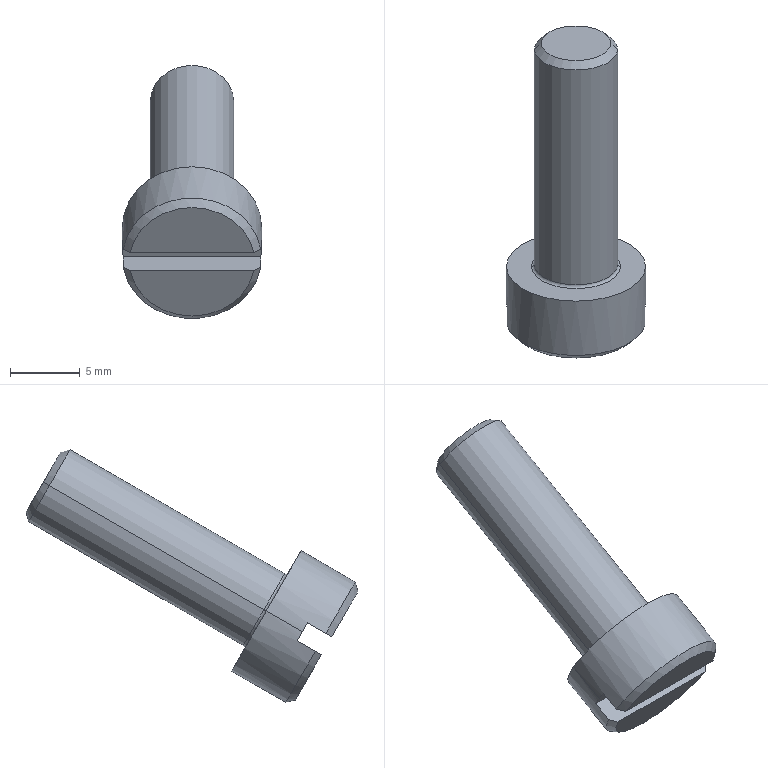Part | SolidWorks | features BaseBody 1 | 1 solid | 17 faces | box 10 x 23.852 x 18.178 mm | volume 880.406 mm3 | plane 7 | cone 4 | cylinder 4 | torus 2 | commonest cylinder face diameters 6 x2 10 x2
STEP:
#1=CARTESIAN_POINT('',(130.5,-22.084,-12.75));
#2=VERTEX_POINT('',#1);
#3=CARTESIAN_POINT('',(135.5,-22.084,-12.75));
#4=VERTEX_POINT('',#3);
#5=CARTESIAN_POINT('',(133.,-22.084,-12.75));
#6=DIRECTION('',(0.,0.866,0.5));
#7=DIRECTION('',(-1.,0.,0.));
#8=AXIS2_PLACEMENT_3D('',#5,#6,#7);
#9=CIRCLE('',#8,2.5);
#10=EDGE_CURVE('',#2,#4,#9,.T.);
#11=ORIENTED_EDGE('',*,*,#10,.F.);
#12=CARTESIAN_POINT('',(130.,-22.517,-13.));
#13=VERTEX_POINT('',#12);
#14=CARTESIAN_POINT('',(130.5,-22.084,-12.75));
#15=DIRECTION('',(-0.7071,-0.6124,-0.3536));
#16=VECTOR('',#15,1000.);
#17=LINE('',#14,#16);
#18=EDGE_CURVE('',#2,#13,#17,.T.);
#19=ORIENTED_EDGE('',*,*,#18,.T.);
#20=CARTESIAN_POINT('',(136.,-22.517,-13.));
#21=VERTEX_POINT('',#20);
#22=CARTESIAN_POINT('',(133.,-22.517,-13.));
#23=DIRECTION('',(0.,-0.866,-0.5));
#24=DIRECTION('',(-1.,0.,0.));
#25=AXIS2_PLACEMENT_3D('',#22,#23,#24);
#26=CIRCLE('',#25,3.);
#27=EDGE_CURVE('',#21,#13,#26,.T.);
#28=ORIENTED_EDGE('',*,*,#27,.F.);
#29=CARTESIAN_POINT('',(135.5,-22.084,-12.75));
#30=DIRECTION('',(0.7071,-0.6124,-0.3536));
#31=VECTOR('',#30,1000.);
#32=LINE('',#29,#31);
#33=EDGE_CURVE('',#4,#21,#32,.T.);
#34=ORIENTED_EDGE('',*,*,#33,.F.);
#35=EDGE_LOOP('',(#11,#19,#28,#34));
#36=FACE_OUTER_BOUND('',#35,.T.);
#37=CARTESIAN_POINT('',(133.,-22.084,-12.75));
#38=DIRECTION('',(0.,-0.866,-0.5));
#39=DIRECTION('',(1.,0.,0.));
#40=AXIS2_PLACEMENT_3D('',#37,#38,#39);
#41=CONICAL_SURFACE('',#40,2.5,0.7854);
#42=ADVANCED_FACE('',(#36),#41,.T.);
#43=CARTESIAN_POINT('',(136.,-37.932,-21.9));
#44=VERTEX_POINT('',#43);
#45=CARTESIAN_POINT('',(130.,-37.932,-21.9));
#46=VERTEX_POINT('',#45);
#47=CARTESIAN_POINT('',(133.,-37.932,-21.9));
#48=DIRECTION('',(0.,0.866,0.5));
#49=DIRECTION('',(-1.,0.,0.));
#50=AXIS2_PLACEMENT_3D('',#47,#48,#49);
#51=CIRCLE('',#50,3.);
#52=EDGE_CURVE('',#44,#46,#51,.T.);
#53=ORIENTED_EDGE('',*,*,#52,.F.);
#54=CARTESIAN_POINT('',(136.2,-38.105,-22.));
#55=VERTEX_POINT('',#54);
#56=CARTESIAN_POINT('',(136.2,-37.932,-21.9));
#57=DIRECTION('',(0.,-0.5,0.866));
#58=DIRECTION('',(0.,-0.866,-0.5));
#59=AXIS2_PLACEMENT_3D('',#56,#57,#58);
#60=CIRCLE('',#59,0.2);
#61=EDGE_CURVE('',#44,#55,#60,.T.);
#62=ORIENTED_EDGE('',*,*,#61,.T.);
#63=CARTESIAN_POINT('',(129.8,-38.105,-22.));
#64=VERTEX_POINT('',#63);
#65=CARTESIAN_POINT('',(133.,-38.105,-22.));
#66=DIRECTION('',(0.,-0.866,-0.5));
#67=DIRECTION('',(-1.,0.,0.));
#68=AXIS2_PLACEMENT_3D('',#65,#66,#67);
#69=CIRCLE('',#68,3.2);
#70=EDGE_CURVE('',#64,#55,#69,.T.);
#71=ORIENTED_EDGE('',*,*,#70,.F.);
#72=CARTESIAN_POINT('',(129.8,-37.932,-21.9));
#73=DIRECTION('',(0.,0.5,-0.866));
#74=DIRECTION('',(0.,0.866,0.5));
#75=AXIS2_PLACEMENT_3D('',#72,#73,#74);
#76=CIRCLE('',#75,0.2);
#77=EDGE_CURVE('',#46,#64,#76,.T.);
#78=ORIENTED_EDGE('',*,*,#77,.F.);
#79=EDGE_LOOP('',(#53,#62,#71,#78));
#80=FACE_OUTER_BOUND('',#79,.T.);
#81=CARTESIAN_POINT('',(133.,-37.932,-21.9));
#82=DIRECTION('',(0.,0.866,0.5));
#83=DIRECTION('',(-1.,0.,0.));
#84=AXIS2_PLACEMENT_3D('',#81,#82,#83);
#85=TOROIDAL_SURFACE('',#84,3.2,0.2);
#86=ADVANCED_FACE('',(#80),#85,.F.);
#87=ORIENTED_EDGE('',*,*,#27,.T.);
#88=CARTESIAN_POINT('',(130.,-22.084,-12.75));
#89=DIRECTION('',(0.,-0.866,-0.5));
#90=VECTOR('',#89,1000.);
#91=LINE('',#88,#90);
#92=EDGE_CURVE('',#13,#46,#91,.T.);
#93=ORIENTED_EDGE('',*,*,#92,.T.);
#94=CARTESIAN_POINT('',(133.,-37.932,-21.9));
#95=DIRECTION('',(0.,0.866,0.5));
#96=DIRECTION('',(-1.,0.,0.));
#97=AXIS2_PLACEMENT_3D('',#94,#95,#96);
#98=CIRCLE('',#97,3.);
#99=EDGE_CURVE('',#46,#44,#98,.T.);
#100=ORIENTED_EDGE('',*,*,#99,.T.);
#101=CARTESIAN_POINT('',(136.,-22.084,-12.75));
#102=DIRECTION('',(0.,-0.866,-0.5));
#103=VECTOR('',#102,1000.);
#104=LINE('',#101,#103);
#105=EDGE_CURVE('',#21,#44,#104,.T.);
#106=ORIENTED_EDGE('',*,*,#105,.F.);
#107=EDGE_LOOP('',(#87,#93,#100,#106));
#108=FACE_OUTER_BOUND('',#107,.T.);
#109=CARTESIAN_POINT('',(133.,-22.084,-12.75));
#110=DIRECTION('',(0.,-0.866,-0.5));
#111=DIRECTION('',(1.,0.,0.));
#112=AXIS2_PLACEMENT_3D('',#109,#110,#111);
#113=CYLINDRICAL_SURFACE('',#112,3.);
#114=ADVANCED_FACE('',(#108),#113,.T.);
#115=CARTESIAN_POINT('',(128.,-38.105,-22.));
#116=VERTEX_POINT('',#115);
#117=CARTESIAN_POINT('',(138.,-38.105,-22.));
#118=VERTEX_POINT('',#117);
#119=CARTESIAN_POINT('',(133.,-38.105,-22.));
#120=DIRECTION('',(0.,0.866,0.5));
#121=DIRECTION('',(-1.,0.,0.));
#122=AXIS2_PLACEMENT_3D('',#119,#120,#121);
#123=CIRCLE('',#122,5.);
#124=EDGE_CURVE('',#116,#118,#123,.T.);
#125=ORIENTED_EDGE('',*,*,#124,.F.);
#126=CARTESIAN_POINT('',(128.,-40.703,-23.5));
#127=VERTEX_POINT('',#126);
#128=CARTESIAN_POINT('',(128.,-38.105,-22.));
#129=DIRECTION('',(0.,-0.866,-0.5));
#130=VECTOR('',#129,1000.);
#131=LINE('',#128,#130);
#132=EDGE_CURVE('',#116,#127,#131,.T.);
#133=ORIENTED_EDGE('',*,*,#132,.T.);
#134=CARTESIAN_POINT('',(128.057,-41.078,-22.85));
#135=VERTEX_POINT('',#134);
#136=CARTESIAN_POINT('',(133.,-40.703,-23.5));
#137=DIRECTION('',(0.,-0.866,-0.5));
#138=DIRECTION('',(1.,0.,0.));
#139=AXIS2_PLACEMENT_3D('',#136,#137,#138);
#140=CIRCLE('',#139,5.);
#141=EDGE_CURVE('',#135,#127,#140,.T.);
#142=ORIENTED_EDGE('',*,*,#141,.F.);
#143=CARTESIAN_POINT('',(128.057,-42.377,-23.6));
#144=VERTEX_POINT('',#143);
#145=CARTESIAN_POINT('',(128.057,-41.078,-22.85));
#146=DIRECTION('',(0.,-0.866,-0.5));
#147=VECTOR('',#146,1000.);
#148=LINE('',#145,#147);
#149=EDGE_CURVE('',#135,#144,#148,.T.);
#150=ORIENTED_EDGE('',*,*,#149,.T.);
#151=CARTESIAN_POINT('',(137.943,-42.377,-23.6));
#152=VERTEX_POINT('',#151);
#153=CARTESIAN_POINT('',(133.,-42.002,-24.25));
#154=DIRECTION('',(0.,0.866,0.5));
#155=DIRECTION('',(-1.,0.,0.));
#156=AXIS2_PLACEMENT_3D('',#153,#154,#155);
#157=CIRCLE('',#156,5.);
#158=EDGE_CURVE('',#144,#152,#157,.T.);
#159=ORIENTED_EDGE('',*,*,#158,.T.);
#160=CARTESIAN_POINT('',(137.943,-41.078,-22.85));
#161=VERTEX_POINT('',#160);
#162=CARTESIAN_POINT('',(137.943,-41.078,-22.85));
#163=DIRECTION('',(0.,-0.866,-0.5));
#164=VECTOR('',#163,1000.);
#165=LINE('',#162,#164);
#166=EDGE_CURVE('',#161,#152,#165,.T.);
#167=ORIENTED_EDGE('',*,*,#166,.F.);
#168=CARTESIAN_POINT('',(138.,-40.703,-23.5));
#169=VERTEX_POINT('',#168);
#170=CARTESIAN_POINT('',(133.,-40.703,-23.5));
#171=DIRECTION('',(0.,-0.866,-0.5));
#172=DIRECTION('',(1.,0.,0.));
#173=AXIS2_PLACEMENT_3D('',#170,#171,#172);
#174=CIRCLE('',#173,5.);
#175=EDGE_CURVE('',#169,#161,#174,.T.);
#176=ORIENTED_EDGE('',*,*,#175,.F.);
#177=CARTESIAN_POINT('',(138.,-38.105,-22.));
#178=DIRECTION('',(0.,-0.866,-0.5));
#179=VECTOR('',#178,1000.);
#180=LINE('',#177,#179);
#181=EDGE_CURVE('',#118,#169,#180,.T.);
#182=ORIENTED_EDGE('',*,*,#181,.F.);
#183=EDGE_LOOP('',(#125,#133,#142,#150,#159,#167,#176,#182));
#184=FACE_OUTER_BOUND('',#183,.T.);
#185=CARTESIAN_POINT('',(133.,-38.105,-22.));
#186=DIRECTION('',(0.,-0.866,-0.5));
#187=DIRECTION('',(1.,0.,0.));
#188=AXIS2_PLACEMENT_3D('',#185,#186,#187);
#189=CYLINDRICAL_SURFACE('',#188,5.);
#190=ADVANCED_FACE('',(#184),#189,.T.);
#191=ORIENTED_EDGE('',*,*,#70,.T.);
#192=CARTESIAN_POINT('',(133.,-38.105,-22.));
#193=DIRECTION('',(0.,-0.866,-0.5));
#194=DIRECTION('',(-1.,0.,0.));
#195=AXIS2_PLACEMENT_3D('',#192,#193,#194);
#196=CIRCLE('',#195,3.2);
#197=EDGE_CURVE('',#55,#64,#196,.T.);
#198=ORIENTED_EDGE('',*,*,#197,.T.);
#199=EDGE_LOOP('',(#191,#198));
#200=FACE_BOUND('',#199,.T.);
#201=CARTESIAN_POINT('',(133.,-38.105,-22.));
#202=DIRECTION('',(0.,0.866,0.5));
#203=DIRECTION('',(-1.,0.,0.));
#204=AXIS2_PLACEMENT_3D('',#201,#202,#203);
#205=CIRCLE('',#204,5.);
#206=EDGE_CURVE('',#118,#116,#205,.T.);
#207=ORIENTED_EDGE('',*,*,#206,.T.);
#208=ORIENTED_EDGE('',*,*,#124,.T.);
#209=EDGE_LOOP('',(#207,#208));
#210=FACE_OUTER_BOUND('',#209,.T.);
#211=CARTESIAN_POINT('',(133.,-38.105,-22.));
#212=DIRECTION('',(0.,0.866,0.5));
#213=DIRECTION('',(-1.,0.,0.));
#214=AXIS2_PLACEMENT_3D('',#211,#212,#213);
#215=PLANE('',#214);
#216=ADVANCED_FACE('',(#200,#210),#215,.T.);
#217=CARTESIAN_POINT('',(137.437,-42.81,-23.85));
#218=VERTEX_POINT('',#217);
#219=CARTESIAN_POINT('',(128.563,-42.81,-23.85));
#220=VERTEX_POINT('',#219);
#221=CARTESIAN_POINT('',(128.057,-42.81,-23.85));
#222=DIRECTION('',(-1.,0.,0.));
#223=VECTOR('',#222,1000.);
#224=LINE('',#221,#223);
#225=EDGE_CURVE('',#218,#220,#224,.T.);
#226=ORIENTED_EDGE('',*,*,#225,.F.);
#227=CARTESIAN_POINT('',(133.,-42.435,-24.5));
#228=DIRECTION('',(0.,-0.866,-0.5));
#229=DIRECTION('',(-1.,0.,0.));
#230=AXIS2_PLACEMENT_3D('',#227,#228,#229);
#231=CIRCLE('',#230,4.5);
#232=EDGE_CURVE('',#218,#220,#231,.T.);
#233=ORIENTED_EDGE('',*,*,#232,.T.);
#234=EDGE_LOOP('',(#226,#233));
#235=FACE_OUTER_BOUND('',#234,.T.);
#236=CARTESIAN_POINT('',(133.,-42.435,-24.5));
#237=DIRECTION('',(0.,0.866,0.5));
#238=DIRECTION('',(-1.,0.,0.));
#239=AXIS2_PLACEMENT_3D('',#236,#237,#238);
#240=PLANE('',#239);
#241=ADVANCED_FACE('',(#235),#240,.F.);
#242=ORIENTED_EDGE('',*,*,#132,.F.);
#243=ORIENTED_EDGE('',*,*,#206,.F.);
#244=ORIENTED_EDGE('',*,*,#181,.T.);
#245=CARTESIAN_POINT('',(137.943,-40.328,-24.15));
#246=VERTEX_POINT('',#245);
#247=CARTESIAN_POINT('',(133.,-40.703,-23.5));
#248=DIRECTION('',(0.,-0.866,-0.5));
#249=DIRECTION('',(1.,0.,0.));
#250=AXIS2_PLACEMENT_3D('',#247,#248,#249);
#251=CIRCLE('',#250,5.);
#252=EDGE_CURVE('',#246,#169,#251,.T.);
#253=ORIENTED_EDGE('',*,*,#252,.F.);
#254=CARTESIAN_POINT('',(137.943,-41.627,-24.9));
#255=VERTEX_POINT('',#254);
#256=CARTESIAN_POINT('',(137.943,-40.328,-24.15));
#257=DIRECTION('',(0.,-0.866,-0.5));
#258=VECTOR('',#257,1000.);
#259=LINE('',#256,#258);
#260=EDGE_CURVE('',#246,#255,#259,.T.);
#261=ORIENTED_EDGE('',*,*,#260,.T.);
#262=CARTESIAN_POINT('',(128.057,-41.627,-24.9));
#263=VERTEX_POINT('',#262);
#264=CARTESIAN_POINT('',(133.,-42.002,-24.25));
#265=DIRECTION('',(0.,0.866,0.5));
#266=DIRECTION('',(-1.,0.,0.));
#267=AXIS2_PLACEMENT_3D('',#264,#265,#266);
#268=CIRCLE('',#267,5.);
#269=EDGE_CURVE('',#255,#263,#268,.T.);
#270=ORIENTED_EDGE('',*,*,#269,.T.);
#271=CARTESIAN_POINT('',(128.057,-40.328,-24.15));
#272=VERTEX_POINT('',#271);
#273=CARTESIAN_POINT('',(128.057,-40.328,-24.15));
#274=DIRECTION('',(0.,-0.866,-0.5));
#275=VECTOR('',#274,1000.);
#276=LINE('',#273,#275);
#277=EDGE_CURVE('',#272,#263,#276,.T.);
#278=ORIENTED_EDGE('',*,*,#277,.F.);
#279=CARTESIAN_POINT('',(133.,-40.703,-23.5));
#280=DIRECTION('',(0.,-0.866,-0.5));
#281=DIRECTION('',(1.,0.,0.));
#282=AXIS2_PLACEMENT_3D('',#279,#280,#281);
#283=CIRCLE('',#282,5.);
#284=EDGE_CURVE('',#127,#272,#283,.T.);
#285=ORIENTED_EDGE('',*,*,#284,.F.);
#286=EDGE_LOOP('',(#242,#243,#244,#253,#261,#270,#278,#285));
#287=FACE_OUTER_BOUND('',#286,.T.);
#288=CARTESIAN_POINT('',(133.,-38.105,-22.));
#289=DIRECTION('',(0.,-0.866,-0.5));
#290=DIRECTION('',(1.,0.,0.));
#291=AXIS2_PLACEMENT_3D('',#288,#289,#290);
#292=CYLINDRICAL_SURFACE('',#291,5.);
#293=ADVANCED_FACE('',(#287),#292,.T.);
#294=CARTESIAN_POINT('',(128.563,-42.06,-25.15));
#295=VERTEX_POINT('',#294);
#296=CARTESIAN_POINT('',(137.437,-42.06,-25.15));
#297=VERTEX_POINT('',#296);
#298=CARTESIAN_POINT('',(128.057,-42.06,-25.15));
#299=DIRECTION('',(1.,0.,0.));
#300=VECTOR('',#299,1000.);
#301=LINE('',#298,#300);
#302=EDGE_CURVE('',#295,#297,#301,.T.);
#303=ORIENTED_EDGE('',*,*,#302,.F.);
#304=CARTESIAN_POINT('',(133.,-42.435,-24.5));
#305=DIRECTION('',(0.,-0.866,-0.5));
#306=DIRECTION('',(-1.,0.,0.));
#307=AXIS2_PLACEMENT_3D('',#304,#305,#306);
#308=CIRCLE('',#307,4.5);
#309=EDGE_CURVE('',#295,#297,#308,.T.);
#310=ORIENTED_EDGE('',*,*,#309,.T.);
#311=EDGE_LOOP('',(#303,#310));
#312=FACE_OUTER_BOUND('',#311,.T.);
#313=CARTESIAN_POINT('',(133.,-42.435,-24.5));
#314=DIRECTION('',(0.,0.866,0.5));
#315=DIRECTION('',(-1.,0.,0.));
#316=AXIS2_PLACEMENT_3D('',#313,#314,#315);
#317=PLANE('',#316);
#318=ADVANCED_FACE('',(#312),#317,.F.);
#319=ORIENTED_EDGE('',*,*,#166,.T.);
#320=CARTESIAN_POINT('',(137.943,-42.377,-23.6));
#321=CARTESIAN_POINT('',(137.775,-42.522,-23.684));
#322=CARTESIAN_POINT('',(137.606,-42.666,-23.767));
#323=CARTESIAN_POINT('',(137.437,-42.81,-23.85));
#324=B_SPLINE_CURVE_WITH_KNOTS('',3,(#320,#321,#322,#323),.UNSPECIFIED.,.F.,.F.,(4,4),(0.,0.0007116),.UNSPECIFIED.);
#325=EDGE_CURVE('',#152,#218,#324,.T.);
#326=ORIENTED_EDGE('',*,*,#325,.T.);
#327=ORIENTED_EDGE('',*,*,#225,.T.);
#328=CARTESIAN_POINT('',(128.563,-42.81,-23.85));
#329=CARTESIAN_POINT('',(128.394,-42.666,-23.767));
#330=CARTESIAN_POINT('',(128.225,-42.522,-23.684));
#331=CARTESIAN_POINT('',(128.057,-42.377,-23.6));
#332=B_SPLINE_CURVE_WITH_KNOTS('',3,(#328,#329,#330,#331),.UNSPECIFIED.,.F.,.F.,(4,4),(0.,0.0007116),.UNSPECIFIED.);
#333=EDGE_CURVE('',#220,#144,#332,.T.);
#334=ORIENTED_EDGE('',*,*,#333,.T.);
#335=ORIENTED_EDGE('',*,*,#149,.F.);
#336=CARTESIAN_POINT('',(128.057,-41.078,-22.85));
#337=DIRECTION('',(-1.,0.,0.));
#338=VECTOR('',#337,1000.);
#339=LINE('',#336,#338);
#340=EDGE_CURVE('',#161,#135,#339,.T.);
#341=ORIENTED_EDGE('',*,*,#340,.F.);
#342=EDGE_LOOP('',(#319,#326,#327,#334,#335,#341));
#343=FACE_OUTER_BOUND('',#342,.T.);
#344=CARTESIAN_POINT('',(128.057,-41.078,-22.85));
#345=DIRECTION('',(0.,-0.5,0.866));
#346=DIRECTION('',(0.,0.866,0.5));
#347=AXIS2_PLACEMENT_3D('',#344,#345,#346);
#348=PLANE('',#347);
#349=ADVANCED_FACE('',(#343),#348,.F.);
#350=ORIENTED_EDGE('',*,*,#277,.T.);
#351=CARTESIAN_POINT('',(128.057,-41.627,-24.9));
#352=CARTESIAN_POINT('',(128.225,-41.772,-24.983));
#353=CARTESIAN_POINT('',(128.394,-41.916,-25.066));
#354=CARTESIAN_POINT('',(128.563,-42.06,-25.15));
#355=B_SPLINE_CURVE_WITH_KNOTS('',3,(#351,#352,#353,#354),.UNSPECIFIED.,.F.,.F.,(4,4),(0.,0.0007116),.UNSPECIFIED.);
#356=EDGE_CURVE('',#263,#295,#355,.T.);
#357=ORIENTED_EDGE('',*,*,#356,.T.);
#358=ORIENTED_EDGE('',*,*,#302,.T.);
#359=CARTESIAN_POINT('',(137.437,-42.06,-25.15));
#360=CARTESIAN_POINT('',(137.606,-41.916,-25.066));
#361=CARTESIAN_POINT('',(137.775,-41.772,-24.983));
#362=CARTESIAN_POINT('',(137.943,-41.627,-24.9));
#363=B_SPLINE_CURVE_WITH_KNOTS('',3,(#359,#360,#361,#362),.UNSPECIFIED.,.F.,.F.,(4,4),(0.,0.0007116),.UNSPECIFIED.);
#364=EDGE_CURVE('',#297,#255,#363,.T.);
#365=ORIENTED_EDGE('',*,*,#364,.T.);
#366=ORIENTED_EDGE('',*,*,#260,.F.);
#367=CARTESIAN_POINT('',(128.057,-40.328,-24.15));
#368=DIRECTION('',(1.,0.,0.));
#369=VECTOR('',#368,1000.);
#370=LINE('',#367,#369);
#371=EDGE_CURVE('',#272,#246,#370,.T.);
#372=ORIENTED_EDGE('',*,*,#371,.F.);
#373=EDGE_LOOP('',(#350,#357,#358,#365,#366,#372));
#374=FACE_OUTER_BOUND('',#373,.T.);
#375=CARTESIAN_POINT('',(128.057,-40.328,-24.15));
#376=DIRECTION('',(0.,0.5,-0.866));
#377=DIRECTION('',(0.,-0.866,-0.5));
#378=AXIS2_PLACEMENT_3D('',#375,#376,#377);
#379=PLANE('',#378);
#380=ADVANCED_FACE('',(#374),#379,.F.);
#381=ORIENTED_EDGE('',*,*,#141,.T.);
#382=ORIENTED_EDGE('',*,*,#284,.T.);
#383=ORIENTED_EDGE('',*,*,#371,.T.);
#384=ORIENTED_EDGE('',*,*,#252,.T.);
#385=ORIENTED_EDGE('',*,*,#175,.T.);
#386=ORIENTED_EDGE('',*,*,#340,.T.);
#387=EDGE_LOOP('',(#381,#382,#383,#384,#385,#386));
#388=FACE_OUTER_BOUND('',#387,.T.);
#389=CARTESIAN_POINT('',(133.,-40.703,-23.5));
#390=DIRECTION('',(0.,-0.866,-0.5));
#391=DIRECTION('',(1.,0.,0.));
#392=AXIS2_PLACEMENT_3D('',#389,#390,#391);
#393=PLANE('',#392);
#394=ADVANCED_FACE('',(#388),#393,.T.);
#395=ORIENTED_EDGE('',*,*,#333,.F.);
#396=ORIENTED_EDGE('',*,*,#232,.F.);
#397=ORIENTED_EDGE('',*,*,#325,.F.);
#398=ORIENTED_EDGE('',*,*,#158,.F.);
#399=EDGE_LOOP('',(#395,#396,#397,#398));
#400=FACE_OUTER_BOUND('',#399,.T.);
#401=CARTESIAN_POINT('',(133.,-42.002,-24.25));
#402=DIRECTION('',(0.,0.866,0.5));
#403=DIRECTION('',(-1.,0.,0.));
#404=AXIS2_PLACEMENT_3D('',#401,#402,#403);
#405=CONICAL_SURFACE('',#404,5.,0.7854);
#406=ADVANCED_FACE('',(#400),#405,.T.);
#407=ORIENTED_EDGE('',*,*,#364,.F.);
#408=ORIENTED_EDGE('',*,*,#309,.F.);
#409=ORIENTED_EDGE('',*,*,#356,.F.);
#410=ORIENTED_EDGE('',*,*,#269,.F.);
#411=EDGE_LOOP('',(#407,#408,#409,#410));
#412=FACE_OUTER_BOUND('',#411,.T.);
#413=CARTESIAN_POINT('',(133.,-42.002,-24.25));
#414=DIRECTION('',(0.,0.866,0.5));
#415=DIRECTION('',(-1.,0.,0.));
#416=AXIS2_PLACEMENT_3D('',#413,#414,#415);
#417=CONICAL_SURFACE('',#416,5.,0.7854);
#418=ADVANCED_FACE('',(#412),#417,.T.);
#419=ORIENTED_EDGE('',*,*,#92,.F.);
#420=CARTESIAN_POINT('',(133.,-22.517,-13.));
#421=DIRECTION('',(0.,-0.866,-0.5));
#422=DIRECTION('',(-1.,0.,0.));
#423=AXIS2_PLACEMENT_3D('',#420,#421,#422);
#424=CIRCLE('',#423,3.);
#425=EDGE_CURVE('',#13,#21,#424,.T.);
#426=ORIENTED_EDGE('',*,*,#425,.T.);
#427=ORIENTED_EDGE('',*,*,#105,.T.);
#428=ORIENTED_EDGE('',*,*,#52,.T.);
#429=EDGE_LOOP('',(#419,#426,#427,#428));
#430=FACE_OUTER_BOUND('',#429,.T.);
#431=CARTESIAN_POINT('',(133.,-22.084,-12.75));
#432=DIRECTION('',(0.,-0.866,-0.5));
#433=DIRECTION('',(1.,0.,0.));
#434=AXIS2_PLACEMENT_3D('',#431,#432,#433);
#435=CYLINDRICAL_SURFACE('',#434,3.);
#436=ADVANCED_FACE('',(#430),#435,.T.);
#437=CARTESIAN_POINT('',(133.,-22.084,-12.75));
#438=DIRECTION('',(0.,0.866,0.5));
#439=DIRECTION('',(-1.,0.,0.));
#440=AXIS2_PLACEMENT_3D('',#437,#438,#439);
#441=CIRCLE('',#440,2.5);
#442=EDGE_CURVE('',#4,#2,#441,.T.);
#443=ORIENTED_EDGE('',*,*,#442,.T.);
#444=ORIENTED_EDGE('',*,*,#10,.T.);
#445=EDGE_LOOP('',(#443,#444));
#446=FACE_OUTER_BOUND('',#445,.T.);
#447=CARTESIAN_POINT('',(133.,-22.084,-12.75));
#448=DIRECTION('',(0.,0.866,0.5));
#449=DIRECTION('',(-1.,0.,0.));
#450=AXIS2_PLACEMENT_3D('',#447,#448,#449);
#451=PLANE('',#450);
#452=ADVANCED_FACE('',(#446),#451,.T.);
#453=ORIENTED_EDGE('',*,*,#61,.F.);
#454=ORIENTED_EDGE('',*,*,#99,.F.);
#455=ORIENTED_EDGE('',*,*,#77,.T.);
#456=ORIENTED_EDGE('',*,*,#197,.F.);
#457=EDGE_LOOP('',(#453,#454,#455,#456));
#458=FACE_OUTER_BOUND('',#457,.T.);
#459=CARTESIAN_POINT('',(133.,-37.932,-21.9));
#460=DIRECTION('',(0.,0.866,0.5));
#461=DIRECTION('',(-1.,0.,0.));
#462=AXIS2_PLACEMENT_3D('',#459,#460,#461);
#463=TOROIDAL_SURFACE('',#462,3.2,0.2);
#464=ADVANCED_FACE('',(#458),#463,.F.);
#465=ORIENTED_EDGE('',*,*,#18,.F.);
#466=ORIENTED_EDGE('',*,*,#442,.F.);
#467=ORIENTED_EDGE('',*,*,#33,.T.);
#468=ORIENTED_EDGE('',*,*,#425,.F.);
#469=EDGE_LOOP('',(#465,#466,#467,#468));
#470=FACE_OUTER_BOUND('',#469,.T.);
#471=CARTESIAN_POINT('',(133.,-22.084,-12.75));
#472=DIRECTION('',(0.,-0.866,-0.5));
#473=DIRECTION('',(1.,0.,0.));
#474=AXIS2_PLACEMENT_3D('',#471,#472,#473);
#475=CONICAL_SURFACE('',#474,2.5,0.7854);
#476=ADVANCED_FACE('',(#470),#475,.T.);
#477=CLOSED_SHELL('',(#42,#86,#114,#190,#216,#241,#293,#318,#349,#380,#394,#406,#418,#436,#452,#464,#476));
#478=MANIFOLD_SOLID_BREP('',#477);
#479=CARTESIAN_POINT('',(0.,0.,0.));
#480=DIRECTION('',(0.,0.,1.));
#481=DIRECTION('',(1.,0.,0.));
#482=AXIS2_PLACEMENT_3D('',#479,#480,#481);
#483=(LENGTH_UNIT()NAMED_UNIT(*)SI_UNIT(.MILLI.,.METRE.));
#484=UNCERTAINTY_MEASURE_WITH_UNIT(LENGTH_MEASURE(0.00001),#483,'','');
#485=(NAMED_UNIT(*)PLANE_ANGLE_UNIT()SI_UNIT($,.RADIAN.));
#486=(NAMED_UNIT(*)SI_UNIT($,.STERADIAN.)SOLID_ANGLE_UNIT());
#487=(GEOMETRIC_REPRESENTATION_CONTEXT(3)GLOBAL_UNCERTAINTY_ASSIGNED_CONTEXT((#484))GLOBAL_UNIT_ASSIGNED_CONTEXT((#483,#485,#486))REPRESENTATION_CONTEXT('',''));
#488=ADVANCED_BREP_SHAPE_REPRESENTATION('',(#478,#482),#487);